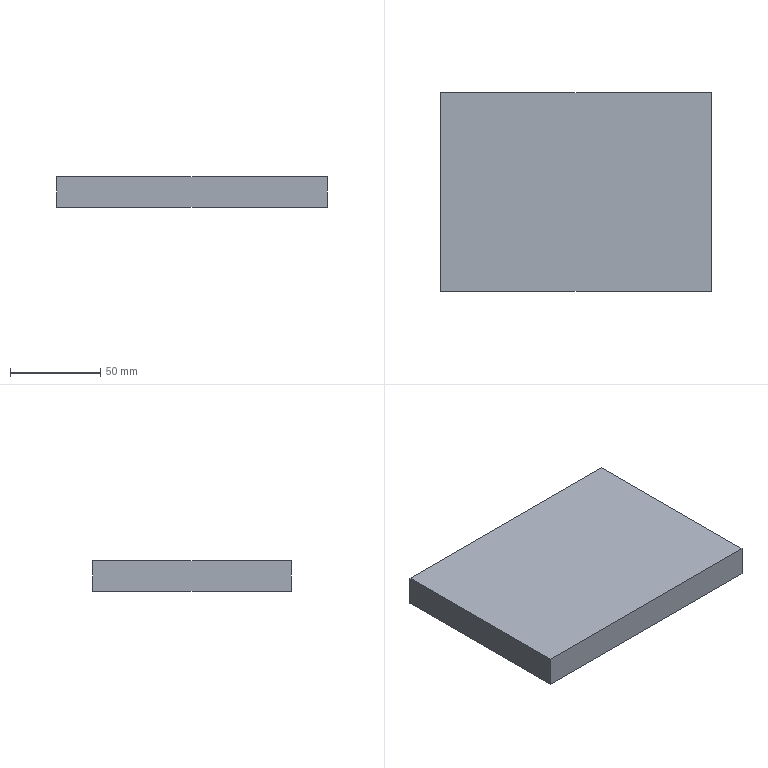Part | STEP file | 1 solid | 6 faces | box 150 x 110 x 17 mm | volume 280500 mm3 | plane 6
STEP:
#1=CARTESIAN_POINT('',(0.,0.,0.));
#2=DIRECTION('',(0.,0.,1.));
#3=DIRECTION('',(1.,0.,0.));
#4=AXIS2_PLACEMENT_3D('',#1,#2,#3);
#5=CARTESIAN_POINT('',(-75.,55.,17.));
#6=VERTEX_POINT('',#5);
#7=CARTESIAN_POINT('',(-75.,-55.,17.));
#8=VERTEX_POINT('',#7);
#9=CARTESIAN_POINT('',(-75.,0.,17.));
#10=DIRECTION('',(0.,-1.,0.));
#11=VECTOR('',#10,1.);
#12=LINE('',#9,#11);
#13=CARTESIAN_POINT('',(0.,0.,17.));
#14=DIRECTION('',(0.,0.,1.));
#15=DIRECTION('',(0.,-1.,0.));
#16=AXIS2_PLACEMENT_3D('',#13,#14,#15);
#17=PLANE('',#16);
#18=CARTESIAN_POINT('',(0.,-75.));
#19=DIRECTION('',(1.,0.));
#20=VECTOR('',#19,1.);
#21=LINE('',#18,#20);
#22=(GEOMETRIC_REPRESENTATION_CONTEXT(2)PARAMETRIC_REPRESENTATION_CONTEXT()REPRESENTATION_CONTEXT('',''));
#23=DEFINITIONAL_REPRESENTATION('',(#21),#22);
#24=PCURVE('',#17,#23);
#25=CARTESIAN_POINT('',(-75.,55.,17.));
#26=DIRECTION('',(1.,0.,0.));
#27=DIRECTION('',(0.,1.,0.));
#28=AXIS2_PLACEMENT_3D('',#25,#26,#27);
#29=PLANE('',#28);
#30=CARTESIAN_POINT('',(-55.,0.));
#31=DIRECTION('',(-1.,0.));
#32=VECTOR('',#31,1.);
#33=LINE('',#30,#32);
#34=(GEOMETRIC_REPRESENTATION_CONTEXT(2)PARAMETRIC_REPRESENTATION_CONTEXT()REPRESENTATION_CONTEXT('',''));
#35=DEFINITIONAL_REPRESENTATION('',(#33),#34);
#36=PCURVE('',#29,#35);
#37=SURFACE_CURVE('',#12,(#24,#36),.PCURVE_S1.);
#38=EDGE_CURVE('',#6,#8,#37,.T.);
#39=ORIENTED_EDGE('',*,*,#38,.T.);
#40=CARTESIAN_POINT('',(75.,-55.,17.));
#41=VERTEX_POINT('',#40);
#42=CARTESIAN_POINT('',(0.,-55.,17.));
#43=DIRECTION('',(1.,0.,0.));
#44=VECTOR('',#43,1.);
#45=LINE('',#42,#44);
#46=CARTESIAN_POINT('',(55.,0.));
#47=DIRECTION('',(0.,1.));
#48=VECTOR('',#47,1.);
#49=LINE('',#46,#48);
#50=(GEOMETRIC_REPRESENTATION_CONTEXT(2)PARAMETRIC_REPRESENTATION_CONTEXT()REPRESENTATION_CONTEXT('',''));
#51=DEFINITIONAL_REPRESENTATION('',(#49),#50);
#52=PCURVE('',#17,#51);
#53=CARTESIAN_POINT('',(-75.,-55.,17.));
#54=DIRECTION('',(0.,1.,0.));
#55=DIRECTION('',(-1.,0.,0.));
#56=AXIS2_PLACEMENT_3D('',#53,#54,#55);
#57=PLANE('',#56);
#58=CARTESIAN_POINT('',(-75.,0.));
#59=DIRECTION('',(-1.,0.));
#60=VECTOR('',#59,1.);
#61=LINE('',#58,#60);
#62=(GEOMETRIC_REPRESENTATION_CONTEXT(2)PARAMETRIC_REPRESENTATION_CONTEXT()REPRESENTATION_CONTEXT('',''));
#63=DEFINITIONAL_REPRESENTATION('',(#61),#62);
#64=PCURVE('',#57,#63);
#65=SURFACE_CURVE('',#45,(#52,#64),.PCURVE_S1.);
#66=EDGE_CURVE('',#8,#41,#65,.T.);
#67=ORIENTED_EDGE('',*,*,#66,.T.);
#68=CARTESIAN_POINT('',(75.,55.,17.));
#69=VERTEX_POINT('',#68);
#70=CARTESIAN_POINT('',(75.,0.,17.));
#71=DIRECTION('',(0.,1.,0.));
#72=VECTOR('',#71,1.);
#73=LINE('',#70,#72);
#74=CARTESIAN_POINT('',(0.,75.));
#75=DIRECTION('',(-1.,0.));
#76=VECTOR('',#75,1.);
#77=LINE('',#74,#76);
#78=(GEOMETRIC_REPRESENTATION_CONTEXT(2)PARAMETRIC_REPRESENTATION_CONTEXT()REPRESENTATION_CONTEXT('',''));
#79=DEFINITIONAL_REPRESENTATION('',(#77),#78);
#80=PCURVE('',#17,#79);
#81=CARTESIAN_POINT('',(75.,55.,17.));
#82=DIRECTION('',(-1.,0.,0.));
#83=DIRECTION('',(0.,-1.,0.));
#84=AXIS2_PLACEMENT_3D('',#81,#82,#83);
#85=PLANE('',#84);
#86=CARTESIAN_POINT('',(55.,0.));
#87=DIRECTION('',(-1.,0.));
#88=VECTOR('',#87,1.);
#89=LINE('',#86,#88);
#90=(GEOMETRIC_REPRESENTATION_CONTEXT(2)PARAMETRIC_REPRESENTATION_CONTEXT()REPRESENTATION_CONTEXT('',''));
#91=DEFINITIONAL_REPRESENTATION('',(#89),#90);
#92=PCURVE('',#85,#91);
#93=SURFACE_CURVE('',#73,(#80,#92),.PCURVE_S1.);
#94=EDGE_CURVE('',#41,#69,#93,.T.);
#95=ORIENTED_EDGE('',*,*,#94,.T.);
#96=CARTESIAN_POINT('',(0.,55.,17.));
#97=DIRECTION('',(-1.,0.,0.));
#98=VECTOR('',#97,1.);
#99=LINE('',#96,#98);
#100=CARTESIAN_POINT('',(-55.,0.));
#101=DIRECTION('',(0.,-1.));
#102=VECTOR('',#101,1.);
#103=LINE('',#100,#102);
#104=(GEOMETRIC_REPRESENTATION_CONTEXT(2)PARAMETRIC_REPRESENTATION_CONTEXT()REPRESENTATION_CONTEXT('',''));
#105=DEFINITIONAL_REPRESENTATION('',(#103),#104);
#106=PCURVE('',#17,#105);
#107=CARTESIAN_POINT('',(-75.,55.,17.));
#108=DIRECTION('',(0.,-1.,0.));
#109=DIRECTION('',(1.,0.,0.));
#110=AXIS2_PLACEMENT_3D('',#107,#108,#109);
#111=PLANE('',#110);
#112=CARTESIAN_POINT('',(75.,0.));
#113=DIRECTION('',(-1.,0.));
#114=VECTOR('',#113,1.);
#115=LINE('',#112,#114);
#116=(GEOMETRIC_REPRESENTATION_CONTEXT(2)PARAMETRIC_REPRESENTATION_CONTEXT()REPRESENTATION_CONTEXT('',''));
#117=DEFINITIONAL_REPRESENTATION('',(#115),#116);
#118=PCURVE('',#111,#117);
#119=SURFACE_CURVE('',#99,(#106,#118),.PCURVE_S1.);
#120=EDGE_CURVE('',#69,#6,#119,.T.);
#121=ORIENTED_EDGE('',*,*,#120,.T.);
#122=EDGE_LOOP('',(#39,#67,#95,#121));
#123=FACE_BOUND('',#122,.T.);
#124=ADVANCED_FACE('',(#123),#17,.T.);
#125=CARTESIAN_POINT('',(75.,-55.,0.));
#126=VERTEX_POINT('',#125);
#127=CARTESIAN_POINT('',(75.,-55.,17.));
#128=DIRECTION('',(0.,0.,-1.));
#129=VECTOR('',#128,1.);
#130=LINE('',#127,#129);
#131=CARTESIAN_POINT('',(-150.,0.));
#132=DIRECTION('',(0.,-1.));
#133=VECTOR('',#132,1.);
#134=LINE('',#131,#133);
#135=(GEOMETRIC_REPRESENTATION_CONTEXT(2)PARAMETRIC_REPRESENTATION_CONTEXT()REPRESENTATION_CONTEXT('',''));
#136=DEFINITIONAL_REPRESENTATION('',(#134),#135);
#137=PCURVE('',#57,#136);
#138=CARTESIAN_POINT('',(110.,0.));
#139=DIRECTION('',(0.,-1.));
#140=VECTOR('',#139,1.);
#141=LINE('',#138,#140);
#142=(GEOMETRIC_REPRESENTATION_CONTEXT(2)PARAMETRIC_REPRESENTATION_CONTEXT()REPRESENTATION_CONTEXT('',''));
#143=DEFINITIONAL_REPRESENTATION('',(#141),#142);
#144=PCURVE('',#85,#143);
#145=SURFACE_CURVE('',#130,(#137,#144),.PCURVE_S1.);
#146=EDGE_CURVE('',#41,#126,#145,.T.);
#147=ORIENTED_EDGE('',*,*,#146,.F.);
#148=ORIENTED_EDGE('',*,*,#66,.F.);
#149=CARTESIAN_POINT('',(-75.,-55.,0.));
#150=VERTEX_POINT('',#149);
#151=CARTESIAN_POINT('',(-75.,-55.,17.));
#152=DIRECTION('',(0.,0.,1.));
#153=VECTOR('',#152,1.);
#154=LINE('',#151,#153);
#155=CARTESIAN_POINT('',(0.,0.));
#156=DIRECTION('',(0.,1.));
#157=VECTOR('',#156,1.);
#158=LINE('',#155,#157);
#159=(GEOMETRIC_REPRESENTATION_CONTEXT(2)PARAMETRIC_REPRESENTATION_CONTEXT()REPRESENTATION_CONTEXT('',''));
#160=DEFINITIONAL_REPRESENTATION('',(#158),#159);
#161=PCURVE('',#57,#160);
#162=CARTESIAN_POINT('',(-110.,0.));
#163=DIRECTION('',(0.,1.));
#164=VECTOR('',#163,1.);
#165=LINE('',#162,#164);
#166=(GEOMETRIC_REPRESENTATION_CONTEXT(2)PARAMETRIC_REPRESENTATION_CONTEXT()REPRESENTATION_CONTEXT('',''));
#167=DEFINITIONAL_REPRESENTATION('',(#165),#166);
#168=PCURVE('',#29,#167);
#169=SURFACE_CURVE('',#154,(#161,#168),.PCURVE_S1.);
#170=EDGE_CURVE('',#150,#8,#169,.T.);
#171=ORIENTED_EDGE('',*,*,#170,.F.);
#172=CARTESIAN_POINT('',(-75.,-55.,0.));
#173=DIRECTION('',(-1.,0.,0.));
#174=VECTOR('',#173,1.);
#175=LINE('',#172,#174);
#176=CARTESIAN_POINT('',(0.,-17.));
#177=DIRECTION('',(1.,0.));
#178=VECTOR('',#177,1.);
#179=LINE('',#176,#178);
#180=(GEOMETRIC_REPRESENTATION_CONTEXT(2)PARAMETRIC_REPRESENTATION_CONTEXT()REPRESENTATION_CONTEXT('',''));
#181=DEFINITIONAL_REPRESENTATION('',(#179),#180);
#182=PCURVE('',#57,#181);
#183=CARTESIAN_POINT('',(0.,0.,0.));
#184=DIRECTION('',(0.,0.,1.));
#185=DIRECTION('',(0.,-1.,0.));
#186=AXIS2_PLACEMENT_3D('',#183,#184,#185);
#187=PLANE('',#186);
#188=CARTESIAN_POINT('',(55.,-75.));
#189=DIRECTION('',(0.,-1.));
#190=VECTOR('',#189,1.);
#191=LINE('',#188,#190);
#192=(GEOMETRIC_REPRESENTATION_CONTEXT(2)PARAMETRIC_REPRESENTATION_CONTEXT()REPRESENTATION_CONTEXT('',''));
#193=DEFINITIONAL_REPRESENTATION('',(#191),#192);
#194=PCURVE('',#187,#193);
#195=SURFACE_CURVE('',#175,(#182,#194),.PCURVE_S1.);
#196=EDGE_CURVE('',#126,#150,#195,.T.);
#197=ORIENTED_EDGE('',*,*,#196,.F.);
#198=EDGE_LOOP('',(#147,#148,#171,#197));
#199=FACE_BOUND('',#198,.T.);
#200=ADVANCED_FACE('',(#199),#57,.F.);
#201=ORIENTED_EDGE('',*,*,#170,.T.);
#202=ORIENTED_EDGE('',*,*,#38,.F.);
#203=CARTESIAN_POINT('',(-75.,55.,0.));
#204=VERTEX_POINT('',#203);
#205=CARTESIAN_POINT('',(-75.,55.,17.));
#206=DIRECTION('',(0.,0.,1.));
#207=VECTOR('',#206,1.);
#208=LINE('',#205,#207);
#209=CARTESIAN_POINT('',(0.,0.));
#210=DIRECTION('',(0.,1.));
#211=VECTOR('',#210,1.);
#212=LINE('',#209,#211);
#213=(GEOMETRIC_REPRESENTATION_CONTEXT(2)PARAMETRIC_REPRESENTATION_CONTEXT()REPRESENTATION_CONTEXT('',''));
#214=DEFINITIONAL_REPRESENTATION('',(#212),#213);
#215=PCURVE('',#29,#214);
#216=CARTESIAN_POINT('',(0.,0.));
#217=DIRECTION('',(0.,1.));
#218=VECTOR('',#217,1.);
#219=LINE('',#216,#218);
#220=(GEOMETRIC_REPRESENTATION_CONTEXT(2)PARAMETRIC_REPRESENTATION_CONTEXT()REPRESENTATION_CONTEXT('',''));
#221=DEFINITIONAL_REPRESENTATION('',(#219),#220);
#222=PCURVE('',#111,#221);
#223=SURFACE_CURVE('',#208,(#215,#222),.PCURVE_S1.);
#224=EDGE_CURVE('',#204,#6,#223,.T.);
#225=ORIENTED_EDGE('',*,*,#224,.F.);
#226=CARTESIAN_POINT('',(-75.,55.,0.));
#227=DIRECTION('',(0.,1.,0.));
#228=VECTOR('',#227,1.);
#229=LINE('',#226,#228);
#230=CARTESIAN_POINT('',(0.,-17.));
#231=DIRECTION('',(1.,0.));
#232=VECTOR('',#231,1.);
#233=LINE('',#230,#232);
#234=(GEOMETRIC_REPRESENTATION_CONTEXT(2)PARAMETRIC_REPRESENTATION_CONTEXT()REPRESENTATION_CONTEXT('',''));
#235=DEFINITIONAL_REPRESENTATION('',(#233),#234);
#236=PCURVE('',#29,#235);
#237=CARTESIAN_POINT('',(-55.,-75.));
#238=DIRECTION('',(-1.,0.));
#239=VECTOR('',#238,1.);
#240=LINE('',#237,#239);
#241=(GEOMETRIC_REPRESENTATION_CONTEXT(2)PARAMETRIC_REPRESENTATION_CONTEXT()REPRESENTATION_CONTEXT('',''));
#242=DEFINITIONAL_REPRESENTATION('',(#240),#241);
#243=PCURVE('',#187,#242);
#244=SURFACE_CURVE('',#229,(#236,#243),.PCURVE_S1.);
#245=EDGE_CURVE('',#150,#204,#244,.T.);
#246=ORIENTED_EDGE('',*,*,#245,.F.);
#247=EDGE_LOOP('',(#201,#202,#225,#246));
#248=FACE_BOUND('',#247,.T.);
#249=ADVANCED_FACE('',(#248),#29,.F.);
#250=ORIENTED_EDGE('',*,*,#224,.T.);
#251=ORIENTED_EDGE('',*,*,#120,.F.);
#252=CARTESIAN_POINT('',(75.,55.,0.));
#253=VERTEX_POINT('',#252);
#254=CARTESIAN_POINT('',(75.,55.,17.));
#255=DIRECTION('',(0.,0.,1.));
#256=VECTOR('',#255,1.);
#257=LINE('',#254,#256);
#258=CARTESIAN_POINT('',(150.,0.));
#259=DIRECTION('',(0.,1.));
#260=VECTOR('',#259,1.);
#261=LINE('',#258,#260);
#262=(GEOMETRIC_REPRESENTATION_CONTEXT(2)PARAMETRIC_REPRESENTATION_CONTEXT()REPRESENTATION_CONTEXT('',''));
#263=DEFINITIONAL_REPRESENTATION('',(#261),#262);
#264=PCURVE('',#111,#263);
#265=CARTESIAN_POINT('',(0.,0.));
#266=DIRECTION('',(0.,1.));
#267=VECTOR('',#266,1.);
#268=LINE('',#265,#267);
#269=(GEOMETRIC_REPRESENTATION_CONTEXT(2)PARAMETRIC_REPRESENTATION_CONTEXT()REPRESENTATION_CONTEXT('',''));
#270=DEFINITIONAL_REPRESENTATION('',(#268),#269);
#271=PCURVE('',#85,#270);
#272=SURFACE_CURVE('',#257,(#264,#271),.PCURVE_S1.);
#273=EDGE_CURVE('',#253,#69,#272,.T.);
#274=ORIENTED_EDGE('',*,*,#273,.F.);
#275=CARTESIAN_POINT('',(-75.,55.,0.));
#276=DIRECTION('',(1.,0.,0.));
#277=VECTOR('',#276,1.);
#278=LINE('',#275,#277);
#279=CARTESIAN_POINT('',(0.,-17.));
#280=DIRECTION('',(1.,0.));
#281=VECTOR('',#280,1.);
#282=LINE('',#279,#281);
#283=(GEOMETRIC_REPRESENTATION_CONTEXT(2)PARAMETRIC_REPRESENTATION_CONTEXT()REPRESENTATION_CONTEXT('',''));
#284=DEFINITIONAL_REPRESENTATION('',(#282),#283);
#285=PCURVE('',#111,#284);
#286=CARTESIAN_POINT('',(-55.,-75.));
#287=DIRECTION('',(0.,1.));
#288=VECTOR('',#287,1.);
#289=LINE('',#286,#288);
#290=(GEOMETRIC_REPRESENTATION_CONTEXT(2)PARAMETRIC_REPRESENTATION_CONTEXT()REPRESENTATION_CONTEXT('',''));
#291=DEFINITIONAL_REPRESENTATION('',(#289),#290);
#292=PCURVE('',#187,#291);
#293=SURFACE_CURVE('',#278,(#285,#292),.PCURVE_S1.);
#294=EDGE_CURVE('',#204,#253,#293,.T.);
#295=ORIENTED_EDGE('',*,*,#294,.F.);
#296=EDGE_LOOP('',(#250,#251,#274,#295));
#297=FACE_BOUND('',#296,.T.);
#298=ADVANCED_FACE('',(#297),#111,.F.);
#299=ORIENTED_EDGE('',*,*,#273,.T.);
#300=ORIENTED_EDGE('',*,*,#94,.F.);
#301=ORIENTED_EDGE('',*,*,#146,.T.);
#302=CARTESIAN_POINT('',(75.,55.,0.));
#303=DIRECTION('',(0.,-1.,0.));
#304=VECTOR('',#303,1.);
#305=LINE('',#302,#304);
#306=CARTESIAN_POINT('',(0.,-17.));
#307=DIRECTION('',(1.,0.));
#308=VECTOR('',#307,1.);
#309=LINE('',#306,#308);
#310=(GEOMETRIC_REPRESENTATION_CONTEXT(2)PARAMETRIC_REPRESENTATION_CONTEXT()REPRESENTATION_CONTEXT('',''));
#311=DEFINITIONAL_REPRESENTATION('',(#309),#310);
#312=PCURVE('',#85,#311);
#313=CARTESIAN_POINT('',(-55.,75.));
#314=DIRECTION('',(1.,0.));
#315=VECTOR('',#314,1.);
#316=LINE('',#313,#315);
#317=(GEOMETRIC_REPRESENTATION_CONTEXT(2)PARAMETRIC_REPRESENTATION_CONTEXT()REPRESENTATION_CONTEXT('',''));
#318=DEFINITIONAL_REPRESENTATION('',(#316),#317);
#319=PCURVE('',#187,#318);
#320=SURFACE_CURVE('',#305,(#312,#319),.PCURVE_S1.);
#321=EDGE_CURVE('',#253,#126,#320,.T.);
#322=ORIENTED_EDGE('',*,*,#321,.F.);
#323=EDGE_LOOP('',(#299,#300,#301,#322));
#324=FACE_BOUND('',#323,.T.);
#325=ADVANCED_FACE('',(#324),#85,.F.);
#326=ORIENTED_EDGE('',*,*,#196,.T.);
#327=ORIENTED_EDGE('',*,*,#245,.T.);
#328=ORIENTED_EDGE('',*,*,#294,.T.);
#329=ORIENTED_EDGE('',*,*,#321,.T.);
#330=EDGE_LOOP('',(#326,#327,#328,#329));
#331=FACE_BOUND('',#330,.T.);
#332=ADVANCED_FACE('',(#331),#187,.F.);
#333=CLOSED_SHELL('',(#124,#200,#249,#298,#325,#332));
#334=MANIFOLD_SOLID_BREP('',#333);
#335=(LENGTH_UNIT()NAMED_UNIT(*)SI_UNIT(.MILLI.,.METRE.));
#336=UNCERTAINTY_MEASURE_WITH_UNIT(LENGTH_MEASURE(0.0000001),#335,'','');
#337=(NAMED_UNIT(*)PLANE_ANGLE_UNIT()SI_UNIT($,.RADIAN.));
#338=(NAMED_UNIT(*)SI_UNIT($,.STERADIAN.)SOLID_ANGLE_UNIT());
#339=(GEOMETRIC_REPRESENTATION_CONTEXT(3)GLOBAL_UNCERTAINTY_ASSIGNED_CONTEXT((#336))GLOBAL_UNIT_ASSIGNED_CONTEXT((#335,#337,#338))REPRESENTATION_CONTEXT('',''));
#340=ADVANCED_BREP_SHAPE_REPRESENTATION('',(#4,#334),#339);